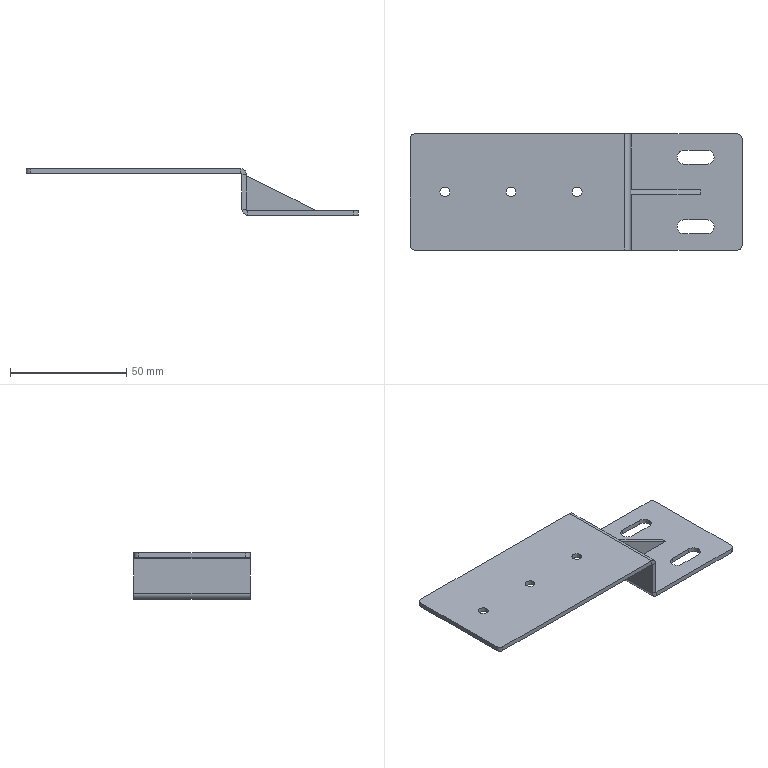Part | SolidWorks | features EdgeFlange 2, Fillet 1, FlatPattern 1, Gusset 1, HoleWzd 1, ICE 1, SMBaseFlange 1, SheetMetal 1 | 2 solids | 47 faces | box 143 x 50 x 20 mm | volume 15978 mm3 | plane 27 | cylinder 20 | commonest cylinder face diameters 4.2 x6 6 x6 4 x4 1 x2 5 x2
STEP:
#1=CARTESIAN_POINT('',(-23.,-1.,15.));
#2=VERTEX_POINT('',#1);
#3=CARTESIAN_POINT('',(7.,-1.,0.));
#4=VERTEX_POINT('',#3);
#5=CARTESIAN_POINT('',(-23.,-1.,15.));
#6=DIRECTION('',(0.8944,0.,-0.4472));
#7=VECTOR('',#6,1000.);
#8=LINE('',#5,#7);
#9=EDGE_CURVE('',#2,#4,#8,.T.);
#10=ORIENTED_EDGE('',*,*,#9,.T.);
#11=CARTESIAN_POINT('',(7.,1.,0.));
#12=VERTEX_POINT('',#11);
#13=CARTESIAN_POINT('',(7.,1.,0.));
#14=DIRECTION('',(0.,-1.,0.));
#15=VECTOR('',#14,1000.);
#16=LINE('',#13,#15);
#17=EDGE_CURVE('',#12,#4,#16,.T.);
#18=ORIENTED_EDGE('',*,*,#17,.F.);
#19=CARTESIAN_POINT('',(-23.,1.,15.));
#20=VERTEX_POINT('',#19);
#21=CARTESIAN_POINT('',(-23.,1.,15.));
#22=DIRECTION('',(0.8944,0.,-0.4472));
#23=VECTOR('',#22,1000.);
#24=LINE('',#21,#23);
#25=EDGE_CURVE('',#20,#12,#24,.T.);
#26=ORIENTED_EDGE('',*,*,#25,.F.);
#27=CARTESIAN_POINT('',(-23.,1.,15.));
#28=DIRECTION('',(0.,-1.,0.));
#29=VECTOR('',#28,1000.);
#30=LINE('',#27,#29);
#31=EDGE_CURVE('',#20,#2,#30,.T.);
#32=ORIENTED_EDGE('',*,*,#31,.T.);
#33=EDGE_LOOP('',(#10,#18,#26,#32));
#34=FACE_OUTER_BOUND('',#33,.T.);
#35=CARTESIAN_POINT('',(-23.,1.,15.));
#36=DIRECTION('',(-0.4472,0.,-0.8944));
#37=DIRECTION('',(-0.8944,0.,0.4472));
#38=AXIS2_PLACEMENT_3D('',#35,#36,#37);
#39=PLANE('',#38);
#40=ADVANCED_FACE('',(#34),#39,.F.);
#41=CARTESIAN_POINT('',(-23.,-1.,0.));
#42=VERTEX_POINT('',#41);
#43=CARTESIAN_POINT('',(-23.,-1.,0.));
#44=DIRECTION('',(-1.,0.,0.));
#45=VECTOR('',#44,1000.);
#46=LINE('',#43,#45);
#47=EDGE_CURVE('',#4,#42,#46,.T.);
#48=ORIENTED_EDGE('',*,*,#47,.T.);
#49=CARTESIAN_POINT('',(-23.,1.,0.));
#50=VERTEX_POINT('',#49);
#51=CARTESIAN_POINT('',(-23.,1.,0.));
#52=DIRECTION('',(0.,-1.,0.));
#53=VECTOR('',#52,1000.);
#54=LINE('',#51,#53);
#55=EDGE_CURVE('',#50,#42,#54,.T.);
#56=ORIENTED_EDGE('',*,*,#55,.F.);
#57=CARTESIAN_POINT('',(-23.,1.,0.));
#58=DIRECTION('',(-1.,0.,0.));
#59=VECTOR('',#58,1000.);
#60=LINE('',#57,#59);
#61=EDGE_CURVE('',#12,#50,#60,.T.);
#62=ORIENTED_EDGE('',*,*,#61,.F.);
#63=ORIENTED_EDGE('',*,*,#17,.T.);
#64=EDGE_LOOP('',(#48,#56,#62,#63));
#65=FACE_OUTER_BOUND('',#64,.T.);
#66=CARTESIAN_POINT('',(-23.,1.,0.));
#67=DIRECTION('',(0.,0.,1.));
#68=DIRECTION('',(1.,0.,0.));
#69=AXIS2_PLACEMENT_3D('',#66,#67,#68);
#70=PLANE('',#69);
#71=ADVANCED_FACE('',(#65),#70,.F.);
#72=CARTESIAN_POINT('',(-23.,-1.,0.));
#73=DIRECTION('',(0.,0.,1.));
#74=VECTOR('',#73,1000.);
#75=LINE('',#72,#74);
#76=EDGE_CURVE('',#42,#2,#75,.T.);
#77=ORIENTED_EDGE('',*,*,#76,.T.);
#78=ORIENTED_EDGE('',*,*,#31,.F.);
#79=CARTESIAN_POINT('',(-23.,1.,0.));
#80=DIRECTION('',(0.,0.,1.));
#81=VECTOR('',#80,1000.);
#82=LINE('',#79,#81);
#83=EDGE_CURVE('',#50,#20,#82,.T.);
#84=ORIENTED_EDGE('',*,*,#83,.F.);
#85=ORIENTED_EDGE('',*,*,#55,.T.);
#86=EDGE_LOOP('',(#77,#78,#84,#85));
#87=FACE_OUTER_BOUND('',#86,.T.);
#88=CARTESIAN_POINT('',(-23.,1.,0.));
#89=DIRECTION('',(1.,0.,0.));
#90=DIRECTION('',(0.,0.,-1.));
#91=AXIS2_PLACEMENT_3D('',#88,#89,#90);
#92=PLANE('',#91);
#93=ADVANCED_FACE('',(#87),#92,.F.);
#94=ORIENTED_EDGE('',*,*,#25,.T.);
#95=ORIENTED_EDGE('',*,*,#61,.T.);
#96=ORIENTED_EDGE('',*,*,#83,.T.);
#97=EDGE_LOOP('',(#94,#95,#96));
#98=FACE_OUTER_BOUND('',#97,.T.);
#99=CARTESIAN_POINT('',(0.,1.,0.));
#100=DIRECTION('',(0.,-1.,0.));
#101=DIRECTION('',(0.,0.,-1.));
#102=AXIS2_PLACEMENT_3D('',#99,#100,#101);
#103=PLANE('',#102);
#104=ADVANCED_FACE('',(#98),#103,.F.);
#105=ORIENTED_EDGE('',*,*,#9,.F.);
#106=ORIENTED_EDGE('',*,*,#76,.F.);
#107=ORIENTED_EDGE('',*,*,#47,.F.);
#108=EDGE_LOOP('',(#105,#106,#107));
#109=FACE_OUTER_BOUND('',#108,.T.);
#110=CARTESIAN_POINT('',(0.,-1.,0.));
#111=DIRECTION('',(0.,-1.,0.));
#112=DIRECTION('',(0.,0.,-1.));
#113=AXIS2_PLACEMENT_3D('',#110,#111,#112);
#114=PLANE('',#113);
#115=ADVANCED_FACE('',(#109),#114,.T.);
#116=CLOSED_SHELL('',(#40,#71,#93,#104,#115));
#117=MANIFOLD_SOLID_BREP('',#116);
#118=CARTESIAN_POINT('',(-105.1,0.,16.));
#119=VERTEX_POINT('',#118);
#120=CARTESIAN_POINT('',(-100.9,0.,16.));
#121=VERTEX_POINT('',#120);
#122=CARTESIAN_POINT('',(-103.,0.,16.));
#123=DIRECTION('',(0.,0.,1.));
#124=DIRECTION('',(1.,0.,0.));
#125=AXIS2_PLACEMENT_3D('',#122,#123,#124);
#126=CIRCLE('',#125,2.1);
#127=EDGE_CURVE('',#119,#121,#126,.T.);
#128=ORIENTED_EDGE('',*,*,#127,.F.);
#129=CARTESIAN_POINT('',(-105.1,0.,18.));
#130=VERTEX_POINT('',#129);
#131=CARTESIAN_POINT('',(-105.1,0.,18.));
#132=DIRECTION('',(0.,0.,1.));
#133=VECTOR('',#132,1000.);
#134=LINE('',#131,#133);
#135=EDGE_CURVE('',#119,#130,#134,.T.);
#136=ORIENTED_EDGE('',*,*,#135,.T.);
#137=CARTESIAN_POINT('',(-100.9,0.,18.));
#138=VERTEX_POINT('',#137);
#139=CARTESIAN_POINT('',(-103.,0.,18.));
#140=DIRECTION('',(0.,0.,1.));
#141=DIRECTION('',(1.,0.,0.));
#142=AXIS2_PLACEMENT_3D('',#139,#140,#141);
#143=CIRCLE('',#142,2.1);
#144=EDGE_CURVE('',#130,#138,#143,.T.);
#145=ORIENTED_EDGE('',*,*,#144,.T.);
#146=CARTESIAN_POINT('',(-100.9,0.,18.));
#147=DIRECTION('',(0.,0.,1.));
#148=VECTOR('',#147,1000.);
#149=LINE('',#146,#148);
#150=EDGE_CURVE('',#121,#138,#149,.T.);
#151=ORIENTED_EDGE('',*,*,#150,.F.);
#152=EDGE_LOOP('',(#128,#136,#145,#151));
#153=FACE_OUTER_BOUND('',#152,.T.);
#154=CARTESIAN_POINT('',(-103.,0.,18.));
#155=DIRECTION('',(0.,0.,1.));
#156=DIRECTION('',(1.,0.,0.));
#157=AXIS2_PLACEMENT_3D('',#154,#155,#156);
#158=CYLINDRICAL_SURFACE('',#157,2.1);
#159=ADVANCED_FACE('',(#153),#158,.F.);
#160=CARTESIAN_POINT('',(-76.6,0.,16.));
#161=VERTEX_POINT('',#160);
#162=CARTESIAN_POINT('',(-72.4,0.,16.));
#163=VERTEX_POINT('',#162);
#164=CARTESIAN_POINT('',(-74.5,0.,16.));
#165=DIRECTION('',(0.,0.,1.));
#166=DIRECTION('',(1.,0.,0.));
#167=AXIS2_PLACEMENT_3D('',#164,#165,#166);
#168=CIRCLE('',#167,2.1);
#169=EDGE_CURVE('',#161,#163,#168,.T.);
#170=ORIENTED_EDGE('',*,*,#169,.F.);
#171=CARTESIAN_POINT('',(-76.6,0.,18.));
#172=VERTEX_POINT('',#171);
#173=CARTESIAN_POINT('',(-76.6,0.,18.));
#174=DIRECTION('',(0.,0.,1.));
#175=VECTOR('',#174,1000.);
#176=LINE('',#173,#175);
#177=EDGE_CURVE('',#161,#172,#176,.T.);
#178=ORIENTED_EDGE('',*,*,#177,.T.);
#179=CARTESIAN_POINT('',(-72.4,0.,18.));
#180=VERTEX_POINT('',#179);
#181=CARTESIAN_POINT('',(-74.5,0.,18.));
#182=DIRECTION('',(0.,0.,1.));
#183=DIRECTION('',(1.,0.,0.));
#184=AXIS2_PLACEMENT_3D('',#181,#182,#183);
#185=CIRCLE('',#184,2.1);
#186=EDGE_CURVE('',#172,#180,#185,.T.);
#187=ORIENTED_EDGE('',*,*,#186,.T.);
#188=CARTESIAN_POINT('',(-72.4,0.,18.));
#189=DIRECTION('',(0.,0.,1.));
#190=VECTOR('',#189,1000.);
#191=LINE('',#188,#190);
#192=EDGE_CURVE('',#163,#180,#191,.T.);
#193=ORIENTED_EDGE('',*,*,#192,.F.);
#194=EDGE_LOOP('',(#170,#178,#187,#193));
#195=FACE_OUTER_BOUND('',#194,.T.);
#196=CARTESIAN_POINT('',(-74.5,0.,18.));
#197=DIRECTION('',(0.,0.,1.));
#198=DIRECTION('',(1.,0.,0.));
#199=AXIS2_PLACEMENT_3D('',#196,#197,#198);
#200=CYLINDRICAL_SURFACE('',#199,2.1);
#201=ADVANCED_FACE('',(#195),#200,.F.);
#202=CARTESIAN_POINT('',(-48.1,0.,16.));
#203=VERTEX_POINT('',#202);
#204=CARTESIAN_POINT('',(-43.9,0.,16.));
#205=VERTEX_POINT('',#204);
#206=CARTESIAN_POINT('',(-46.,0.,16.));
#207=DIRECTION('',(0.,0.,1.));
#208=DIRECTION('',(1.,0.,0.));
#209=AXIS2_PLACEMENT_3D('',#206,#207,#208);
#210=CIRCLE('',#209,2.1);
#211=EDGE_CURVE('',#203,#205,#210,.T.);
#212=ORIENTED_EDGE('',*,*,#211,.F.);
#213=CARTESIAN_POINT('',(-48.1,0.,18.));
#214=VERTEX_POINT('',#213);
#215=CARTESIAN_POINT('',(-48.1,0.,18.));
#216=DIRECTION('',(0.,0.,1.));
#217=VECTOR('',#216,1000.);
#218=LINE('',#215,#217);
#219=EDGE_CURVE('',#203,#214,#218,.T.);
#220=ORIENTED_EDGE('',*,*,#219,.T.);
#221=CARTESIAN_POINT('',(-43.9,0.,18.));
#222=VERTEX_POINT('',#221);
#223=CARTESIAN_POINT('',(-46.,0.,18.));
#224=DIRECTION('',(0.,0.,1.));
#225=DIRECTION('',(1.,0.,0.));
#226=AXIS2_PLACEMENT_3D('',#223,#224,#225);
#227=CIRCLE('',#226,2.1);
#228=EDGE_CURVE('',#214,#222,#227,.T.);
#229=ORIENTED_EDGE('',*,*,#228,.T.);
#230=CARTESIAN_POINT('',(-43.9,0.,18.));
#231=DIRECTION('',(0.,0.,1.));
#232=VECTOR('',#231,1000.);
#233=LINE('',#230,#232);
#234=EDGE_CURVE('',#205,#222,#233,.T.);
#235=ORIENTED_EDGE('',*,*,#234,.F.);
#236=EDGE_LOOP('',(#212,#220,#229,#235));
#237=FACE_OUTER_BOUND('',#236,.T.);
#238=CARTESIAN_POINT('',(-46.,0.,18.));
#239=DIRECTION('',(0.,0.,1.));
#240=DIRECTION('',(1.,0.,0.));
#241=AXIS2_PLACEMENT_3D('',#238,#239,#240);
#242=CYLINDRICAL_SURFACE('',#241,2.1);
#243=ADVANCED_FACE('',(#237),#242,.F.);
#244=CARTESIAN_POINT('',(10.,-12.,-2.));
#245=VERTEX_POINT('',#244);
#246=CARTESIAN_POINT('',(13.,-15.,-2.));
#247=VERTEX_POINT('',#246);
#248=CARTESIAN_POINT('',(10.,-15.,-2.));
#249=DIRECTION('',(0.,0.,-1.));
#250=DIRECTION('',(1.,0.,0.));
#251=AXIS2_PLACEMENT_3D('',#248,#249,#250);
#252=CIRCLE('',#251,3.);
#253=EDGE_CURVE('',#245,#247,#252,.T.);
#254=ORIENTED_EDGE('',*,*,#253,.T.);
#255=CARTESIAN_POINT('',(13.,-15.,0.));
#256=VERTEX_POINT('',#255);
#257=CARTESIAN_POINT('',(13.,-15.,-2.001));
#258=DIRECTION('',(0.,0.,1.));
#259=VECTOR('',#258,1000.);
#260=LINE('',#257,#259);
#261=EDGE_CURVE('',#247,#256,#260,.T.);
#262=ORIENTED_EDGE('',*,*,#261,.T.);
#263=CARTESIAN_POINT('',(10.,-12.,0.));
#264=VERTEX_POINT('',#263);
#265=CARTESIAN_POINT('',(10.,-15.,0.));
#266=DIRECTION('',(0.,0.,1.));
#267=DIRECTION('',(1.,0.,0.));
#268=AXIS2_PLACEMENT_3D('',#265,#266,#267);
#269=CIRCLE('',#268,3.);
#270=EDGE_CURVE('',#256,#264,#269,.T.);
#271=ORIENTED_EDGE('',*,*,#270,.T.);
#272=CARTESIAN_POINT('',(10.,-12.,-2.001));
#273=DIRECTION('',(0.,0.,1.));
#274=VECTOR('',#273,1000.);
#275=LINE('',#272,#274);
#276=EDGE_CURVE('',#245,#264,#275,.T.);
#277=ORIENTED_EDGE('',*,*,#276,.F.);
#278=EDGE_LOOP('',(#254,#262,#271,#277));
#279=FACE_OUTER_BOUND('',#278,.T.);
#280=CARTESIAN_POINT('',(10.,-15.,-2.001));
#281=DIRECTION('',(0.,0.,1.));
#282=DIRECTION('',(1.,0.,0.));
#283=AXIS2_PLACEMENT_3D('',#280,#281,#282);
#284=CYLINDRICAL_SURFACE('',#283,3.);
#285=ADVANCED_FACE('',(#279),#284,.F.);
#286=CARTESIAN_POINT('',(10.,18.,-2.));
#287=VERTEX_POINT('',#286);
#288=CARTESIAN_POINT('',(13.,15.,-2.));
#289=VERTEX_POINT('',#288);
#290=CARTESIAN_POINT('',(10.,15.,-2.));
#291=DIRECTION('',(0.,0.,-1.));
#292=DIRECTION('',(1.,0.,0.));
#293=AXIS2_PLACEMENT_3D('',#290,#291,#292);
#294=CIRCLE('',#293,3.);
#295=EDGE_CURVE('',#287,#289,#294,.T.);
#296=ORIENTED_EDGE('',*,*,#295,.T.);
#297=CARTESIAN_POINT('',(13.,15.,0.));
#298=VERTEX_POINT('',#297);
#299=CARTESIAN_POINT('',(13.,15.,-2.001));
#300=DIRECTION('',(0.,0.,1.));
#301=VECTOR('',#300,1000.);
#302=LINE('',#299,#301);
#303=EDGE_CURVE('',#289,#298,#302,.T.);
#304=ORIENTED_EDGE('',*,*,#303,.T.);
#305=CARTESIAN_POINT('',(10.,18.,0.));
#306=VERTEX_POINT('',#305);
#307=CARTESIAN_POINT('',(10.,15.,0.));
#308=DIRECTION('',(0.,0.,1.));
#309=DIRECTION('',(1.,0.,0.));
#310=AXIS2_PLACEMENT_3D('',#307,#308,#309);
#311=CIRCLE('',#310,3.);
#312=EDGE_CURVE('',#298,#306,#311,.T.);
#313=ORIENTED_EDGE('',*,*,#312,.T.);
#314=CARTESIAN_POINT('',(10.,18.,-2.001));
#315=DIRECTION('',(0.,0.,1.));
#316=VECTOR('',#315,1000.);
#317=LINE('',#314,#316);
#318=EDGE_CURVE('',#287,#306,#317,.T.);
#319=ORIENTED_EDGE('',*,*,#318,.F.);
#320=EDGE_LOOP('',(#296,#304,#313,#319));
#321=FACE_OUTER_BOUND('',#320,.T.);
#322=CARTESIAN_POINT('',(10.,15.,-2.001));
#323=DIRECTION('',(0.,0.,1.));
#324=DIRECTION('',(1.,0.,0.));
#325=AXIS2_PLACEMENT_3D('',#322,#323,#324);
#326=CYLINDRICAL_SURFACE('',#325,3.);
#327=ADVANCED_FACE('',(#321),#326,.F.);
#328=CARTESIAN_POINT('',(-25.,25.,15.5));
#329=VERTEX_POINT('',#328);
#330=CARTESIAN_POINT('',(-23.,25.,15.5));
#331=VERTEX_POINT('',#330);
#332=CARTESIAN_POINT('',(-25.,25.,15.5));
#333=DIRECTION('',(1.,0.,0.));
#334=VECTOR('',#333,1000.);
#335=LINE('',#332,#334);
#336=EDGE_CURVE('',#329,#331,#335,.T.);
#337=ORIENTED_EDGE('',*,*,#336,.T.);
#338=CARTESIAN_POINT('',(-23.,25.,0.5));
#339=VERTEX_POINT('',#338);
#340=CARTESIAN_POINT('',(-23.,25.,0.));
#341=DIRECTION('',(0.,0.,-1.));
#342=VECTOR('',#341,1000.);
#343=LINE('',#340,#342);
#344=EDGE_CURVE('',#331,#339,#343,.T.);
#345=ORIENTED_EDGE('',*,*,#344,.T.);
#346=CARTESIAN_POINT('',(-25.,25.,0.5));
#347=VERTEX_POINT('',#346);
#348=CARTESIAN_POINT('',(-25.,25.,0.5));
#349=DIRECTION('',(-1.,0.,0.));
#350=VECTOR('',#349,1000.);
#351=LINE('',#348,#350);
#352=EDGE_CURVE('',#339,#347,#351,.T.);
#353=ORIENTED_EDGE('',*,*,#352,.T.);
#354=CARTESIAN_POINT('',(-25.,25.,0.));
#355=DIRECTION('',(0.,0.,-1.));
#356=VECTOR('',#355,1000.);
#357=LINE('',#354,#356);
#358=EDGE_CURVE('',#329,#347,#357,.T.);
#359=ORIENTED_EDGE('',*,*,#358,.F.);
#360=EDGE_LOOP('',(#337,#345,#353,#359));
#361=FACE_OUTER_BOUND('',#360,.T.);
#362=CARTESIAN_POINT('',(-25.,25.,0.));
#363=DIRECTION('',(0.,-1.,0.));
#364=DIRECTION('',(0.,0.,-1.));
#365=AXIS2_PLACEMENT_3D('',#362,#363,#364);
#366=PLANE('',#365);
#367=ADVANCED_FACE('',(#361),#366,.F.);
#368=CARTESIAN_POINT('',(-25.,-25.,15.5));
#369=VERTEX_POINT('',#368);
#370=CARTESIAN_POINT('',(-23.,-25.,15.5));
#371=VERTEX_POINT('',#370);
#372=CARTESIAN_POINT('',(-25.,-25.,15.5));
#373=DIRECTION('',(1.,0.,0.));
#374=VECTOR('',#373,1000.);
#375=LINE('',#372,#374);
#376=EDGE_CURVE('',#369,#371,#375,.T.);
#377=ORIENTED_EDGE('',*,*,#376,.F.);
#378=CARTESIAN_POINT('',(-25.,-25.,0.5));
#379=VERTEX_POINT('',#378);
#380=CARTESIAN_POINT('',(-25.,-25.,0.));
#381=DIRECTION('',(0.,0.,1.));
#382=VECTOR('',#381,1000.);
#383=LINE('',#380,#382);
#384=EDGE_CURVE('',#379,#369,#383,.T.);
#385=ORIENTED_EDGE('',*,*,#384,.F.);
#386=CARTESIAN_POINT('',(-23.,-25.,0.5));
#387=VERTEX_POINT('',#386);
#388=CARTESIAN_POINT('',(-23.,-25.,0.5));
#389=DIRECTION('',(-1.,0.,0.));
#390=VECTOR('',#389,1000.);
#391=LINE('',#388,#390);
#392=EDGE_CURVE('',#387,#379,#391,.T.);
#393=ORIENTED_EDGE('',*,*,#392,.F.);
#394=CARTESIAN_POINT('',(-23.,-25.,18.));
#395=DIRECTION('',(0.,0.,1.));
#396=VECTOR('',#395,1000.);
#397=LINE('',#394,#396);
#398=EDGE_CURVE('',#387,#371,#397,.T.);
#399=ORIENTED_EDGE('',*,*,#398,.T.);
#400=EDGE_LOOP('',(#377,#385,#393,#399));
#401=FACE_OUTER_BOUND('',#400,.T.);
#402=CARTESIAN_POINT('',(-25.,-25.,18.));
#403=DIRECTION('',(0.,1.,0.));
#404=DIRECTION('',(0.,0.,1.));
#405=AXIS2_PLACEMENT_3D('',#402,#403,#404);
#406=PLANE('',#405);
#407=ADVANCED_FACE('',(#401),#406,.F.);
#408=CARTESIAN_POINT('',(-25.,25.,15.5));
#409=DIRECTION('',(0.,-1.,0.));
#410=VECTOR('',#409,1000.);
#411=LINE('',#408,#410);
#412=EDGE_CURVE('',#329,#369,#411,.T.);
#413=ORIENTED_EDGE('',*,*,#412,.F.);
#414=ORIENTED_EDGE('',*,*,#358,.T.);
#415=CARTESIAN_POINT('',(-25.,25.,0.5));
#416=DIRECTION('',(0.,1.,0.));
#417=VECTOR('',#416,1000.);
#418=LINE('',#415,#417);
#419=EDGE_CURVE('',#379,#347,#418,.T.);
#420=ORIENTED_EDGE('',*,*,#419,.F.);
#421=ORIENTED_EDGE('',*,*,#384,.T.);
#422=EDGE_LOOP('',(#413,#414,#420,#421));
#423=FACE_OUTER_BOUND('',#422,.T.);
#424=CARTESIAN_POINT('',(-25.,0.,0.));
#425=DIRECTION('',(1.,0.,0.));
#426=DIRECTION('',(0.,0.,-1.));
#427=AXIS2_PLACEMENT_3D('',#424,#425,#426);
#428=PLANE('',#427);
#429=ADVANCED_FACE('',(#423),#428,.F.);
#430=ORIENTED_EDGE('',*,*,#344,.F.);
#431=CARTESIAN_POINT('',(-23.,25.,15.5));
#432=DIRECTION('',(0.,-1.,0.));
#433=VECTOR('',#432,1000.);
#434=LINE('',#431,#433);
#435=EDGE_CURVE('',#331,#371,#434,.T.);
#436=ORIENTED_EDGE('',*,*,#435,.T.);
#437=ORIENTED_EDGE('',*,*,#398,.F.);
#438=CARTESIAN_POINT('',(-23.,25.,0.5));
#439=DIRECTION('',(0.,-1.,0.));
#440=VECTOR('',#439,1000.);
#441=LINE('',#438,#440);
#442=EDGE_CURVE('',#339,#387,#441,.T.);
#443=ORIENTED_EDGE('',*,*,#442,.F.);
#444=EDGE_LOOP('',(#430,#436,#437,#443));
#445=FACE_OUTER_BOUND('',#444,.T.);
#446=CARTESIAN_POINT('',(-23.,0.,0.));
#447=DIRECTION('',(1.,0.,0.));
#448=DIRECTION('',(0.,0.,-1.));
#449=AXIS2_PLACEMENT_3D('',#446,#447,#448);
#450=PLANE('',#449);
#451=ADVANCED_FACE('',(#445),#450,.T.);
#452=CARTESIAN_POINT('',(-22.5,-25.,-2.));
#453=VERTEX_POINT('',#452);
#454=CARTESIAN_POINT('',(23.,-25.,-2.));
#455=VERTEX_POINT('',#454);
#456=CARTESIAN_POINT('',(25.,-25.,-2.));
#457=DIRECTION('',(1.,0.,0.));
#458=VECTOR('',#457,1000.);
#459=LINE('',#456,#458);
#460=EDGE_CURVE('',#453,#455,#459,.T.);
#461=ORIENTED_EDGE('',*,*,#460,.T.);
#462=CARTESIAN_POINT('',(23.,-25.,0.));
#463=VERTEX_POINT('',#462);
#464=CARTESIAN_POINT('',(23.,-25.,-2.));
#465=DIRECTION('',(0.,0.,1.));
#466=VECTOR('',#465,1000.);
#467=LINE('',#464,#466);
#468=EDGE_CURVE('',#455,#463,#467,.T.);
#469=ORIENTED_EDGE('',*,*,#468,.T.);
#470=CARTESIAN_POINT('',(-22.5,-25.,0.));
#471=VERTEX_POINT('',#470);
#472=CARTESIAN_POINT('',(25.,-25.,0.));
#473=DIRECTION('',(1.,0.,0.));
#474=VECTOR('',#473,1000.);
#475=LINE('',#472,#474);
#476=EDGE_CURVE('',#471,#463,#475,.T.);
#477=ORIENTED_EDGE('',*,*,#476,.F.);
#478=CARTESIAN_POINT('',(-22.5,-25.,0.));
#479=DIRECTION('',(0.,0.,-1.));
#480=VECTOR('',#479,1000.);
#481=LINE('',#478,#480);
#482=EDGE_CURVE('',#471,#453,#481,.T.);
#483=ORIENTED_EDGE('',*,*,#482,.T.);
#484=EDGE_LOOP('',(#461,#469,#477,#483));
#485=FACE_OUTER_BOUND('',#484,.T.);
#486=CARTESIAN_POINT('',(25.,-25.,-2.));
#487=DIRECTION('',(0.,-1.,0.));
#488=DIRECTION('',(0.,0.,-1.));
#489=AXIS2_PLACEMENT_3D('',#486,#487,#488);
#490=PLANE('',#489);
#491=ADVANCED_FACE('',(#485),#490,.T.);
#492=CARTESIAN_POINT('',(0.,-12.,-2.));
#493=VERTEX_POINT('',#492);
#494=CARTESIAN_POINT('',(0.,-12.,-2.));
#495=DIRECTION('',(1.,0.,0.));
#496=VECTOR('',#495,1000.);
#497=LINE('',#494,#496);
#498=EDGE_CURVE('',#493,#245,#497,.T.);
#499=ORIENTED_EDGE('',*,*,#498,.F.);
#500=CARTESIAN_POINT('',(0.,-18.,-2.));
#501=VERTEX_POINT('',#500);
#502=CARTESIAN_POINT('',(0.,-15.,-2.));
#503=DIRECTION('',(0.,0.,-1.));
#504=DIRECTION('',(1.,0.,0.));
#505=AXIS2_PLACEMENT_3D('',#502,#503,#504);
#506=CIRCLE('',#505,3.);
#507=EDGE_CURVE('',#501,#493,#506,.T.);
#508=ORIENTED_EDGE('',*,*,#507,.F.);
#509=CARTESIAN_POINT('',(10.,-18.,-2.));
#510=VERTEX_POINT('',#509);
#511=CARTESIAN_POINT('',(0.,-18.,-2.));
#512=DIRECTION('',(-1.,0.,0.));
#513=VECTOR('',#512,1000.);
#514=LINE('',#511,#513);
#515=EDGE_CURVE('',#510,#501,#514,.T.);
#516=ORIENTED_EDGE('',*,*,#515,.F.);
#517=CARTESIAN_POINT('',(10.,-15.,-2.));
#518=DIRECTION('',(0.,0.,-1.));
#519=DIRECTION('',(1.,0.,0.));
#520=AXIS2_PLACEMENT_3D('',#517,#518,#519);
#521=CIRCLE('',#520,3.);
#522=EDGE_CURVE('',#247,#510,#521,.T.);
#523=ORIENTED_EDGE('',*,*,#522,.F.);
#524=ORIENTED_EDGE('',*,*,#253,.F.);
#525=EDGE_LOOP('',(#499,#508,#516,#523,#524));
#526=FACE_BOUND('',#525,.T.);
#527=CARTESIAN_POINT('',(0.,18.,-2.));
#528=VERTEX_POINT('',#527);
#529=CARTESIAN_POINT('',(0.,18.,-2.));
#530=DIRECTION('',(1.,0.,0.));
#531=VECTOR('',#530,1000.);
#532=LINE('',#529,#531);
#533=EDGE_CURVE('',#528,#287,#532,.T.);
#534=ORIENTED_EDGE('',*,*,#533,.F.);
#535=CARTESIAN_POINT('',(0.,12.,-2.));
#536=VERTEX_POINT('',#535);
#537=CARTESIAN_POINT('',(0.,15.,-2.));
#538=DIRECTION('',(0.,0.,-1.));
#539=DIRECTION('',(1.,0.,0.));
#540=AXIS2_PLACEMENT_3D('',#537,#538,#539);
#541=CIRCLE('',#540,3.);
#542=EDGE_CURVE('',#536,#528,#541,.T.);
#543=ORIENTED_EDGE('',*,*,#542,.F.);
#544=CARTESIAN_POINT('',(10.,12.,-2.));
#545=VERTEX_POINT('',#544);
#546=CARTESIAN_POINT('',(0.,12.,-2.));
#547=DIRECTION('',(-1.,0.,0.));
#548=VECTOR('',#547,1000.);
#549=LINE('',#546,#548);
#550=EDGE_CURVE('',#545,#536,#549,.T.);
#551=ORIENTED_EDGE('',*,*,#550,.F.);
#552=CARTESIAN_POINT('',(10.,15.,-2.));
#553=DIRECTION('',(0.,0.,-1.));
#554=DIRECTION('',(1.,0.,0.));
#555=AXIS2_PLACEMENT_3D('',#552,#553,#554);
#556=CIRCLE('',#555,3.);
#557=EDGE_CURVE('',#289,#545,#556,.T.);
#558=ORIENTED_EDGE('',*,*,#557,.F.);
#559=ORIENTED_EDGE('',*,*,#295,.F.);
#560=EDGE_LOOP('',(#534,#543,#551,#558,#559));
#561=FACE_BOUND('',#560,.T.);
#562=CARTESIAN_POINT('',(25.,-23.,-2.));
#563=VERTEX_POINT('',#562);
#564=CARTESIAN_POINT('',(25.,23.,-2.));
#565=VERTEX_POINT('',#564);
#566=CARTESIAN_POINT('',(25.,-25.,-2.));
#567=DIRECTION('',(0.,1.,0.));
#568=VECTOR('',#567,1000.);
#569=LINE('',#566,#568);
#570=EDGE_CURVE('',#563,#565,#569,.T.);
#571=ORIENTED_EDGE('',*,*,#570,.F.);
#572=CARTESIAN_POINT('',(23.,-23.,-2.));
#573=DIRECTION('',(0.,0.,-1.));
#574=DIRECTION('',(1.,0.,0.));
#575=AXIS2_PLACEMENT_3D('',#572,#573,#574);
#576=CIRCLE('',#575,2.);
#577=EDGE_CURVE('',#563,#455,#576,.T.);
#578=ORIENTED_EDGE('',*,*,#577,.T.);
#579=ORIENTED_EDGE('',*,*,#460,.F.);
#580=CARTESIAN_POINT('',(-22.5,25.,-2.));
#581=VERTEX_POINT('',#580);
#582=CARTESIAN_POINT('',(-22.5,-25.,-2.));
#583=DIRECTION('',(0.,1.,0.));
#584=VECTOR('',#583,1000.);
#585=LINE('',#582,#584);
#586=EDGE_CURVE('',#453,#581,#585,.T.);
#587=ORIENTED_EDGE('',*,*,#586,.T.);
#588=CARTESIAN_POINT('',(23.,25.,-2.));
#589=VERTEX_POINT('',#588);
#590=CARTESIAN_POINT('',(25.,25.,-2.));
#591=DIRECTION('',(-1.,0.,0.));
#592=VECTOR('',#591,1000.);
#593=LINE('',#590,#592);
#594=EDGE_CURVE('',#589,#581,#593,.T.);
#595=ORIENTED_EDGE('',*,*,#594,.F.);
#596=CARTESIAN_POINT('',(23.,23.,-2.));
#597=DIRECTION('',(0.,0.,-1.));
#598=DIRECTION('',(1.,0.,0.));
#599=AXIS2_PLACEMENT_3D('',#596,#597,#598);
#600=CIRCLE('',#599,2.);
#601=EDGE_CURVE('',#589,#565,#600,.T.);
#602=ORIENTED_EDGE('',*,*,#601,.T.);
#603=EDGE_LOOP('',(#571,#578,#579,#587,#595,#602));
#604=FACE_OUTER_BOUND('',#603,.T.);
#605=CARTESIAN_POINT('',(0.,0.,-2.));
#606=DIRECTION('',(0.,0.,1.));
#607=DIRECTION('',(1.,0.,0.));
#608=AXIS2_PLACEMENT_3D('',#605,#606,#607);
#609=PLANE('',#608);
#610=ADVANCED_FACE('',(#526,#561,#604),#609,.F.);
#611=CARTESIAN_POINT('',(0.,-12.,0.));
#612=VERTEX_POINT('',#611);
#613=CARTESIAN_POINT('',(0.,-18.,0.));
#614=VERTEX_POINT('',#613);
#615=CARTESIAN_POINT('',(0.,-15.,0.));
#616=DIRECTION('',(0.,0.,1.));
#617=DIRECTION('',(1.,0.,0.));
#618=AXIS2_PLACEMENT_3D('',#615,#616,#617);
#619=CIRCLE('',#618,3.);
#620=EDGE_CURVE('',#612,#614,#619,.T.);
#621=ORIENTED_EDGE('',*,*,#620,.F.);
#622=CARTESIAN_POINT('',(0.,-12.,0.));
#623=DIRECTION('',(-1.,0.,0.));
#624=VECTOR('',#623,1000.);
#625=LINE('',#622,#624);
#626=EDGE_CURVE('',#264,#612,#625,.T.);
#627=ORIENTED_EDGE('',*,*,#626,.F.);
#628=ORIENTED_EDGE('',*,*,#270,.F.);
#629=CARTESIAN_POINT('',(10.,-18.,0.));
#630=VERTEX_POINT('',#629);
#631=CARTESIAN_POINT('',(10.,-15.,0.));
#632=DIRECTION('',(0.,0.,1.));
#633=DIRECTION('',(1.,0.,0.));
#634=AXIS2_PLACEMENT_3D('',#631,#632,#633);
#635=CIRCLE('',#634,3.);
#636=EDGE_CURVE('',#630,#256,#635,.T.);
#637=ORIENTED_EDGE('',*,*,#636,.F.);
#638=CARTESIAN_POINT('',(0.,-18.,0.));
#639=DIRECTION('',(1.,0.,0.));
#640=VECTOR('',#639,1000.);
#641=LINE('',#638,#640);
#642=EDGE_CURVE('',#614,#630,#641,.T.);
#643=ORIENTED_EDGE('',*,*,#642,.F.);
#644=EDGE_LOOP('',(#621,#627,#628,#637,#643));
#645=FACE_BOUND('',#644,.T.);
#646=CARTESIAN_POINT('',(0.,18.,0.));
#647=VERTEX_POINT('',#646);
#648=CARTESIAN_POINT('',(0.,12.,0.));
#649=VERTEX_POINT('',#648);
#650=CARTESIAN_POINT('',(0.,15.,0.));
#651=DIRECTION('',(0.,0.,1.));
#652=DIRECTION('',(1.,0.,0.));
#653=AXIS2_PLACEMENT_3D('',#650,#651,#652);
#654=CIRCLE('',#653,3.);
#655=EDGE_CURVE('',#647,#649,#654,.T.);
#656=ORIENTED_EDGE('',*,*,#655,.F.);
#657=CARTESIAN_POINT('',(0.,18.,0.));
#658=DIRECTION('',(-1.,0.,0.));
#659=VECTOR('',#658,1000.);
#660=LINE('',#657,#659);
#661=EDGE_CURVE('',#306,#647,#660,.T.);
#662=ORIENTED_EDGE('',*,*,#661,.F.);
#663=ORIENTED_EDGE('',*,*,#312,.F.);
#664=CARTESIAN_POINT('',(10.,12.,0.));
#665=VERTEX_POINT('',#664);
#666=CARTESIAN_POINT('',(10.,15.,0.));
#667=DIRECTION('',(0.,0.,1.));
#668=DIRECTION('',(1.,0.,0.));
#669=AXIS2_PLACEMENT_3D('',#666,#667,#668);
#670=CIRCLE('',#669,3.);
#671=EDGE_CURVE('',#665,#298,#670,.T.);
#672=ORIENTED_EDGE('',*,*,#671,.F.);
#673=CARTESIAN_POINT('',(0.,12.,0.));
#674=DIRECTION('',(1.,0.,0.));
#675=VECTOR('',#674,1000.);
#676=LINE('',#673,#675);
#677=EDGE_CURVE('',#649,#665,#676,.T.);
#678=ORIENTED_EDGE('',*,*,#677,.F.);
#679=EDGE_LOOP('',(#656,#662,#663,#672,#678));
#680=FACE_BOUND('',#679,.T.);
#681=ORIENTED_EDGE('',*,*,#476,.T.);
#682=CARTESIAN_POINT('',(25.,-23.,0.));
#683=VERTEX_POINT('',#682);
#684=CARTESIAN_POINT('',(23.,-23.,0.));
#685=DIRECTION('',(0.,0.,1.));
#686=DIRECTION('',(1.,0.,0.));
#687=AXIS2_PLACEMENT_3D('',#684,#685,#686);
#688=CIRCLE('',#687,2.);
#689=EDGE_CURVE('',#463,#683,#688,.T.);
#690=ORIENTED_EDGE('',*,*,#689,.T.);
#691=CARTESIAN_POINT('',(25.,23.,0.));
#692=VERTEX_POINT('',#691);
#693=CARTESIAN_POINT('',(25.,-25.,0.));
#694=DIRECTION('',(0.,1.,0.));
#695=VECTOR('',#694,1000.);
#696=LINE('',#693,#695);
#697=EDGE_CURVE('',#683,#692,#696,.T.);
#698=ORIENTED_EDGE('',*,*,#697,.T.);
#699=CARTESIAN_POINT('',(23.,25.,0.));
#700=VERTEX_POINT('',#699);
#701=CARTESIAN_POINT('',(23.,23.,0.));
#702=DIRECTION('',(0.,0.,1.));
#703=DIRECTION('',(1.,0.,0.));
#704=AXIS2_PLACEMENT_3D('',#701,#702,#703);
#705=CIRCLE('',#704,2.);
#706=EDGE_CURVE('',#692,#700,#705,.T.);
#707=ORIENTED_EDGE('',*,*,#706,.T.);
#708=CARTESIAN_POINT('',(-22.5,25.,0.));
#709=VERTEX_POINT('',#708);
#710=CARTESIAN_POINT('',(25.,25.,0.));
#711=DIRECTION('',(-1.,0.,0.));
#712=VECTOR('',#711,1000.);
#713=LINE('',#710,#712);
#714=EDGE_CURVE('',#700,#709,#713,.T.);
#715=ORIENTED_EDGE('',*,*,#714,.T.);
#716=CARTESIAN_POINT('',(-22.5,-25.,0.));
#717=DIRECTION('',(0.,1.,0.));
#718=VECTOR('',#717,1000.);
#719=LINE('',#716,#718);
#720=EDGE_CURVE('',#471,#709,#719,.T.);
#721=ORIENTED_EDGE('',*,*,#720,.F.);
#722=EDGE_LOOP('',(#681,#690,#698,#707,#715,#721));
#723=FACE_OUTER_BOUND('',#722,.T.);
#724=CARTESIAN_POINT('',(0.,0.,0.));
#725=DIRECTION('',(0.,0.,1.));
#726=DIRECTION('',(1.,0.,0.));
#727=AXIS2_PLACEMENT_3D('',#724,#725,#726);
#728=PLANE('',#727);
#729=ADVANCED_FACE('',(#645,#680,#723),#728,.T.);
#730=ORIENTED_EDGE('',*,*,#714,.F.);
#731=CARTESIAN_POINT('',(23.,25.,-2.));
#732=DIRECTION('',(0.,0.,-1.));
#733=VECTOR('',#732,1000.);
#734=LINE('',#731,#733);
#735=EDGE_CURVE('',#700,#589,#734,.T.);
#736=ORIENTED_EDGE('',*,*,#735,.T.);
#737=ORIENTED_EDGE('',*,*,#594,.T.);
#738=CARTESIAN_POINT('',(-22.5,25.,0.));
#739=DIRECTION('',(0.,0.,-1.));
#740=VECTOR('',#739,1000.);
#741=LINE('',#738,#740);
#742=EDGE_CURVE('',#709,#581,#741,.T.);
#743=ORIENTED_EDGE('',*,*,#742,.F.);
#744=EDGE_LOOP('',(#730,#736,#737,#743));
#745=FACE_OUTER_BOUND('',#744,.T.);
#746=CARTESIAN_POINT('',(25.,25.,-2.));
#747=DIRECTION('',(0.,1.,0.));
#748=DIRECTION('',(0.,0.,1.));
#749=AXIS2_PLACEMENT_3D('',#746,#747,#748);
#750=PLANE('',#749);
#751=ADVANCED_FACE('',(#745),#750,.T.);
#752=ORIENTED_EDGE('',*,*,#697,.F.);
#753=CARTESIAN_POINT('',(25.,-23.,-2.));
#754=DIRECTION('',(0.,0.,-1.));
#755=VECTOR('',#754,1000.);
#756=LINE('',#753,#755);
#757=EDGE_CURVE('',#683,#563,#756,.T.);
#758=ORIENTED_EDGE('',*,*,#757,.T.);
#759=ORIENTED_EDGE('',*,*,#570,.T.);
#760=CARTESIAN_POINT('',(25.,23.,-2.));
#761=DIRECTION('',(0.,0.,1.));
#762=VECTOR('',#761,1000.);
#763=LINE('',#760,#762);
#764=EDGE_CURVE('',#565,#692,#763,.T.);
#765=ORIENTED_EDGE('',*,*,#764,.T.);
#766=EDGE_LOOP('',(#752,#758,#759,#765));
#767=FACE_OUTER_BOUND('',#766,.T.);
#768=CARTESIAN_POINT('',(25.,-25.,-2.));
#769=DIRECTION('',(1.,0.,0.));
#770=DIRECTION('',(0.,0.,-1.));
#771=AXIS2_PLACEMENT_3D('',#768,#769,#770);
#772=PLANE('',#771);
#773=ADVANCED_FACE('',(#767),#772,.T.);
#774=ORIENTED_EDGE('',*,*,#352,.F.);
#775=CARTESIAN_POINT('',(-22.5,25.,0.5));
#776=DIRECTION('',(0.,1.,0.));
#777=DIRECTION('',(0.,0.,-1.));
#778=AXIS2_PLACEMENT_3D('',#775,#776,#777);
#779=CIRCLE('',#778,0.5);
#780=EDGE_CURVE('',#709,#339,#779,.T.);
#781=ORIENTED_EDGE('',*,*,#780,.F.);
#782=ORIENTED_EDGE('',*,*,#742,.T.);
#783=CARTESIAN_POINT('',(-22.5,25.,0.5));
#784=DIRECTION('',(0.,1.,0.));
#785=DIRECTION('',(0.,0.,-1.));
#786=AXIS2_PLACEMENT_3D('',#783,#784,#785);
#787=CIRCLE('',#786,2.5);
#788=EDGE_CURVE('',#581,#347,#787,.T.);
#789=ORIENTED_EDGE('',*,*,#788,.T.);
#790=EDGE_LOOP('',(#774,#781,#782,#789));
#791=FACE_OUTER_BOUND('',#790,.T.);
#792=CARTESIAN_POINT('',(-22.5,25.,0.5));
#793=DIRECTION('',(0.,1.,0.));
#794=DIRECTION('',(0.,0.,1.));
#795=AXIS2_PLACEMENT_3D('',#792,#793,#794);
#796=PLANE('',#795);
#797=ADVANCED_FACE('',(#791),#796,.T.);
#798=CARTESIAN_POINT('',(-22.5,-25.,0.5));
#799=DIRECTION('',(0.,-1.,0.));
#800=DIRECTION('',(0.,0.,-1.));
#801=AXIS2_PLACEMENT_3D('',#798,#799,#800);
#802=CIRCLE('',#801,0.5);
#803=EDGE_CURVE('',#387,#471,#802,.T.);
#804=ORIENTED_EDGE('',*,*,#803,.F.);
#805=ORIENTED_EDGE('',*,*,#392,.T.);
#806=CARTESIAN_POINT('',(-22.5,-25.,0.5));
#807=DIRECTION('',(0.,-1.,0.));
#808=DIRECTION('',(0.,0.,-1.));
#809=AXIS2_PLACEMENT_3D('',#806,#807,#808);
#810=CIRCLE('',#809,2.5);
#811=EDGE_CURVE('',#379,#453,#810,.T.);
#812=ORIENTED_EDGE('',*,*,#811,.T.);
#813=ORIENTED_EDGE('',*,*,#482,.F.);
#814=EDGE_LOOP('',(#804,#805,#812,#813));
#815=FACE_OUTER_BOUND('',#814,.T.);
#816=CARTESIAN_POINT('',(-22.5,-25.,0.5));
#817=DIRECTION('',(0.,1.,0.));
#818=DIRECTION('',(0.,0.,1.));
#819=AXIS2_PLACEMENT_3D('',#816,#817,#818);
#820=PLANE('',#819);
#821=ADVANCED_FACE('',(#815),#820,.F.);
#822=ORIENTED_EDGE('',*,*,#586,.F.);
#823=ORIENTED_EDGE('',*,*,#811,.F.);
#824=ORIENTED_EDGE('',*,*,#419,.T.);
#825=ORIENTED_EDGE('',*,*,#788,.F.);
#826=EDGE_LOOP('',(#822,#823,#824,#825));
#827=FACE_OUTER_BOUND('',#826,.T.);
#828=CARTESIAN_POINT('',(-22.5,-25.,0.5));
#829=DIRECTION('',(0.,-1.,0.));
#830=DIRECTION('',(-1.,0.,0.));
#831=AXIS2_PLACEMENT_3D('',#828,#829,#830);
#832=CYLINDRICAL_SURFACE('',#831,2.5);
#833=ADVANCED_FACE('',(#827),#832,.T.);
#834=ORIENTED_EDGE('',*,*,#720,.T.);
#835=ORIENTED_EDGE('',*,*,#780,.T.);
#836=ORIENTED_EDGE('',*,*,#442,.T.);
#837=ORIENTED_EDGE('',*,*,#803,.T.);
#838=EDGE_LOOP('',(#834,#835,#836,#837));
#839=FACE_OUTER_BOUND('',#838,.T.);
#840=CARTESIAN_POINT('',(-22.5,-25.,0.5));
#841=DIRECTION('',(0.,-1.,0.));
#842=DIRECTION('',(-1.,0.,0.));
#843=AXIS2_PLACEMENT_3D('',#840,#841,#842);
#844=CYLINDRICAL_SURFACE('',#843,0.5);
#845=ADVANCED_FACE('',(#839),#844,.F.);
#846=CARTESIAN_POINT('',(-25.5,-25.,16.));
#847=VERTEX_POINT('',#846);
#848=CARTESIAN_POINT('',(-25.5,-25.,18.));
#849=VERTEX_POINT('',#848);
#850=CARTESIAN_POINT('',(-25.5,-25.,18.));
#851=DIRECTION('',(0.,0.,1.));
#852=VECTOR('',#851,1000.);
#853=LINE('',#850,#852);
#854=EDGE_CURVE('',#847,#849,#853,.T.);
#855=ORIENTED_EDGE('',*,*,#854,.F.);
#856=CARTESIAN_POINT('',(-25.5,-25.,15.5));
#857=DIRECTION('',(0.,-1.,0.));
#858=DIRECTION('',(0.,0.,1.));
#859=AXIS2_PLACEMENT_3D('',#856,#857,#858);
#860=CIRCLE('',#859,0.5);
#861=EDGE_CURVE('',#369,#847,#860,.T.);
#862=ORIENTED_EDGE('',*,*,#861,.F.);
#863=ORIENTED_EDGE('',*,*,#376,.T.);
#864=CARTESIAN_POINT('',(-25.5,-25.,15.5));
#865=DIRECTION('',(0.,-1.,0.));
#866=DIRECTION('',(0.,0.,1.));
#867=AXIS2_PLACEMENT_3D('',#864,#865,#866);
#868=CIRCLE('',#867,2.5);
#869=EDGE_CURVE('',#371,#849,#868,.T.);
#870=ORIENTED_EDGE('',*,*,#869,.T.);
#871=EDGE_LOOP('',(#855,#862,#863,#870));
#872=FACE_OUTER_BOUND('',#871,.T.);
#873=CARTESIAN_POINT('',(-25.5,-25.,15.5));
#874=DIRECTION('',(0.,-1.,0.));
#875=DIRECTION('',(0.,0.,-1.));
#876=AXIS2_PLACEMENT_3D('',#873,#874,#875);
#877=PLANE('',#876);
#878=ADVANCED_FACE('',(#872),#877,.T.);
#879=CARTESIAN_POINT('',(-25.5,25.,16.));
#880=VERTEX_POINT('',#879);
#881=CARTESIAN_POINT('',(-25.5,25.,15.5));
#882=DIRECTION('',(0.,1.,0.));
#883=DIRECTION('',(0.,0.,1.));
#884=AXIS2_PLACEMENT_3D('',#881,#882,#883);
#885=CIRCLE('',#884,0.5);
#886=EDGE_CURVE('',#880,#329,#885,.T.);
#887=ORIENTED_EDGE('',*,*,#886,.F.);
#888=CARTESIAN_POINT('',(-25.5,25.,18.));
#889=VERTEX_POINT('',#888);
#890=CARTESIAN_POINT('',(-25.5,25.,16.));
#891=DIRECTION('',(0.,0.,1.));
#892=VECTOR('',#891,1000.);
#893=LINE('',#890,#892);
#894=EDGE_CURVE('',#880,#889,#893,.T.);
#895=ORIENTED_EDGE('',*,*,#894,.T.);
#896=CARTESIAN_POINT('',(-25.5,25.,15.5));
#897=DIRECTION('',(0.,1.,0.));
#898=DIRECTION('',(0.,0.,1.));
#899=AXIS2_PLACEMENT_3D('',#896,#897,#898);
#900=CIRCLE('',#899,2.5);
#901=EDGE_CURVE('',#889,#331,#900,.T.);
#902=ORIENTED_EDGE('',*,*,#901,.T.);
#903=ORIENTED_EDGE('',*,*,#336,.F.);
#904=EDGE_LOOP('',(#887,#895,#902,#903));
#905=FACE_OUTER_BOUND('',#904,.T.);
#906=CARTESIAN_POINT('',(-25.5,25.,15.5));
#907=DIRECTION('',(0.,-1.,0.));
#908=DIRECTION('',(0.,0.,-1.));
#909=AXIS2_PLACEMENT_3D('',#906,#907,#908);
#910=PLANE('',#909);
#911=ADVANCED_FACE('',(#905),#910,.F.);
#912=ORIENTED_EDGE('',*,*,#435,.F.);
#913=ORIENTED_EDGE('',*,*,#901,.F.);
#914=CARTESIAN_POINT('',(-25.5,0.,18.));
#915=DIRECTION('',(0.,1.,0.));
#916=VECTOR('',#915,1000.);
#917=LINE('',#914,#916);
#918=EDGE_CURVE('',#849,#889,#917,.T.);
#919=ORIENTED_EDGE('',*,*,#918,.F.);
#920=ORIENTED_EDGE('',*,*,#869,.F.);
#921=EDGE_LOOP('',(#912,#913,#919,#920));
#922=FACE_OUTER_BOUND('',#921,.T.);
#923=CARTESIAN_POINT('',(-25.5,25.,15.5));
#924=DIRECTION('',(0.,1.,0.));
#925=DIRECTION('',(0.,0.,1.));
#926=AXIS2_PLACEMENT_3D('',#923,#924,#925);
#927=CYLINDRICAL_SURFACE('',#926,2.5);
#928=ADVANCED_FACE('',(#922),#927,.T.);
#929=ORIENTED_EDGE('',*,*,#412,.T.);
#930=ORIENTED_EDGE('',*,*,#861,.T.);
#931=CARTESIAN_POINT('',(-25.5,-25.,16.));
#932=DIRECTION('',(0.,1.,0.));
#933=VECTOR('',#932,1000.);
#934=LINE('',#931,#933);
#935=EDGE_CURVE('',#847,#880,#934,.T.);
#936=ORIENTED_EDGE('',*,*,#935,.T.);
#937=ORIENTED_EDGE('',*,*,#886,.T.);
#938=EDGE_LOOP('',(#929,#930,#936,#937));
#939=FACE_OUTER_BOUND('',#938,.T.);
#940=CARTESIAN_POINT('',(-25.5,25.,15.5));
#941=DIRECTION('',(0.,1.,0.));
#942=DIRECTION('',(0.,0.,1.));
#943=AXIS2_PLACEMENT_3D('',#940,#941,#942);
#944=CYLINDRICAL_SURFACE('',#943,0.5);
#945=ADVANCED_FACE('',(#939),#944,.F.);
#946=CARTESIAN_POINT('',(-116.,25.,16.));
#947=VERTEX_POINT('',#946);
#948=CARTESIAN_POINT('',(0.,25.,16.));
#949=DIRECTION('',(1.,0.,0.));
#950=VECTOR('',#949,1000.);
#951=LINE('',#948,#950);
#952=EDGE_CURVE('',#947,#880,#951,.T.);
#953=ORIENTED_EDGE('',*,*,#952,.F.);
#954=CARTESIAN_POINT('',(-116.,25.,18.));
#955=VERTEX_POINT('',#954);
#956=CARTESIAN_POINT('',(-116.,25.,18.));
#957=DIRECTION('',(0.,0.,1.));
#958=VECTOR('',#957,1000.);
#959=LINE('',#956,#958);
#960=EDGE_CURVE('',#947,#955,#959,.T.);
#961=ORIENTED_EDGE('',*,*,#960,.T.);
#962=CARTESIAN_POINT('',(-25.,25.,18.));
#963=DIRECTION('',(1.,0.,0.));
#964=VECTOR('',#963,1000.);
#965=LINE('',#962,#964);
#966=EDGE_CURVE('',#955,#889,#965,.T.);
#967=ORIENTED_EDGE('',*,*,#966,.T.);
#968=ORIENTED_EDGE('',*,*,#894,.F.);
#969=EDGE_LOOP('',(#953,#961,#967,#968));
#970=FACE_OUTER_BOUND('',#969,.T.);
#971=CARTESIAN_POINT('',(-25.,25.,18.));
#972=DIRECTION('',(0.,1.,0.));
#973=DIRECTION('',(0.,0.,1.));
#974=AXIS2_PLACEMENT_3D('',#971,#972,#973);
#975=PLANE('',#974);
#976=ADVANCED_FACE('',(#970),#975,.T.);
#977=CARTESIAN_POINT('',(-116.,-25.,18.));
#978=VERTEX_POINT('',#977);
#979=CARTESIAN_POINT('',(-118.,-25.,18.));
#980=DIRECTION('',(-1.,0.,0.));
#981=VECTOR('',#980,1000.);
#982=LINE('',#979,#981);
#983=EDGE_CURVE('',#849,#978,#982,.T.);
#984=ORIENTED_EDGE('',*,*,#983,.T.);
#985=CARTESIAN_POINT('',(-116.,-25.,16.));
#986=VERTEX_POINT('',#985);
#987=CARTESIAN_POINT('',(-116.,-25.,18.));
#988=DIRECTION('',(0.,0.,-1.));
#989=VECTOR('',#988,1000.);
#990=LINE('',#987,#989);
#991=EDGE_CURVE('',#978,#986,#990,.T.);
#992=ORIENTED_EDGE('',*,*,#991,.T.);
#993=CARTESIAN_POINT('',(0.,-25.,16.));
#994=DIRECTION('',(-1.,0.,0.));
#995=VECTOR('',#994,1000.);
#996=LINE('',#993,#995);
#997=EDGE_CURVE('',#847,#986,#996,.T.);
#998=ORIENTED_EDGE('',*,*,#997,.F.);
#999=ORIENTED_EDGE('',*,*,#854,.T.);
#1000=EDGE_LOOP('',(#984,#992,#998,#999));
#1001=FACE_OUTER_BOUND('',#1000,.T.);
#1002=CARTESIAN_POINT('',(-118.,-25.,18.));
#1003=DIRECTION('',(0.,-1.,0.));
#1004=DIRECTION('',(0.,0.,-1.));
#1005=AXIS2_PLACEMENT_3D('',#1002,#1003,#1004);
#1006=PLANE('',#1005);
#1007=ADVANCED_FACE('',(#1001),#1006,.T.);
#1008=CARTESIAN_POINT('',(-103.,0.,18.));
#1009=DIRECTION('',(0.,0.,1.));
#1010=DIRECTION('',(1.,0.,0.));
#1011=AXIS2_PLACEMENT_3D('',#1008,#1009,#1010);
#1012=CIRCLE('',#1011,2.1);
#1013=EDGE_CURVE('',#138,#130,#1012,.T.);
#1014=ORIENTED_EDGE('',*,*,#1013,.F.);
#1015=ORIENTED_EDGE('',*,*,#144,.F.);
#1016=EDGE_LOOP('',(#1014,#1015));
#1017=FACE_BOUND('',#1016,.T.);
#1018=CARTESIAN_POINT('',(-74.5,0.,18.));
#1019=DIRECTION('',(0.,0.,1.));
#1020=DIRECTION('',(1.,0.,0.));
#1021=AXIS2_PLACEMENT_3D('',#1018,#1019,#1020);
#1022=CIRCLE('',#1021,2.1);
#1023=EDGE_CURVE('',#180,#172,#1022,.T.);
#1024=ORIENTED_EDGE('',*,*,#1023,.F.);
#1025=ORIENTED_EDGE('',*,*,#186,.F.);
#1026=EDGE_LOOP('',(#1024,#1025));
#1027=FACE_BOUND('',#1026,.T.);
#1028=CARTESIAN_POINT('',(-46.,0.,18.));
#1029=DIRECTION('',(0.,0.,1.));
#1030=DIRECTION('',(1.,0.,0.));
#1031=AXIS2_PLACEMENT_3D('',#1028,#1029,#1030);
#1032=CIRCLE('',#1031,2.1);
#1033=EDGE_CURVE('',#222,#214,#1032,.T.);
#1034=ORIENTED_EDGE('',*,*,#1033,.F.);
#1035=ORIENTED_EDGE('',*,*,#228,.F.);
#1036=EDGE_LOOP('',(#1034,#1035));
#1037=FACE_BOUND('',#1036,.T.);
#1038=ORIENTED_EDGE('',*,*,#966,.F.);
#1039=CARTESIAN_POINT('',(-118.,23.,18.));
#1040=VERTEX_POINT('',#1039);
#1041=CARTESIAN_POINT('',(-116.,23.,18.));
#1042=DIRECTION('',(0.,0.,1.));
#1043=DIRECTION('',(1.,0.,0.));
#1044=AXIS2_PLACEMENT_3D('',#1041,#1042,#1043);
#1045=CIRCLE('',#1044,2.);
#1046=EDGE_CURVE('',#955,#1040,#1045,.T.);
#1047=ORIENTED_EDGE('',*,*,#1046,.T.);
#1048=CARTESIAN_POINT('',(-118.,-23.,18.));
#1049=VERTEX_POINT('',#1048);
#1050=CARTESIAN_POINT('',(-118.,25.,18.));
#1051=DIRECTION('',(0.,1.,0.));
#1052=VECTOR('',#1051,1000.);
#1053=LINE('',#1050,#1052);
#1054=EDGE_CURVE('',#1049,#1040,#1053,.T.);
#1055=ORIENTED_EDGE('',*,*,#1054,.F.);
#1056=CARTESIAN_POINT('',(-116.,-23.,18.));
#1057=DIRECTION('',(0.,0.,1.));
#1058=DIRECTION('',(1.,0.,0.));
#1059=AXIS2_PLACEMENT_3D('',#1056,#1057,#1058);
#1060=CIRCLE('',#1059,2.);
#1061=EDGE_CURVE('',#1049,#978,#1060,.T.);
#1062=ORIENTED_EDGE('',*,*,#1061,.T.);
#1063=ORIENTED_EDGE('',*,*,#983,.F.);
#1064=ORIENTED_EDGE('',*,*,#918,.T.);
#1065=EDGE_LOOP('',(#1038,#1047,#1055,#1062,#1063,#1064));
#1066=FACE_OUTER_BOUND('',#1065,.T.);
#1067=CARTESIAN_POINT('',(0.,0.,18.));
#1068=DIRECTION('',(0.,0.,1.));
#1069=DIRECTION('',(1.,0.,0.));
#1070=AXIS2_PLACEMENT_3D('',#1067,#1068,#1069);
#1071=PLANE('',#1070);
#1072=ADVANCED_FACE('',(#1017,#1027,#1037,#1066),#1071,.T.);
#1073=CARTESIAN_POINT('',(-103.,0.,16.));
#1074=DIRECTION('',(0.,0.,1.));
#1075=DIRECTION('',(1.,0.,0.));
#1076=AXIS2_PLACEMENT_3D('',#1073,#1074,#1075);
#1077=CIRCLE('',#1076,2.1);
#1078=EDGE_CURVE('',#121,#119,#1077,.T.);
#1079=ORIENTED_EDGE('',*,*,#1078,.T.);
#1080=ORIENTED_EDGE('',*,*,#127,.T.);
#1081=EDGE_LOOP('',(#1079,#1080));
#1082=FACE_BOUND('',#1081,.T.);
#1083=CARTESIAN_POINT('',(-74.5,0.,16.));
#1084=DIRECTION('',(0.,0.,1.));
#1085=DIRECTION('',(1.,0.,0.));
#1086=AXIS2_PLACEMENT_3D('',#1083,#1084,#1085);
#1087=CIRCLE('',#1086,2.1);
#1088=EDGE_CURVE('',#163,#161,#1087,.T.);
#1089=ORIENTED_EDGE('',*,*,#1088,.T.);
#1090=ORIENTED_EDGE('',*,*,#169,.T.);
#1091=EDGE_LOOP('',(#1089,#1090));
#1092=FACE_BOUND('',#1091,.T.);
#1093=CARTESIAN_POINT('',(-46.,0.,16.));
#1094=DIRECTION('',(0.,0.,1.));
#1095=DIRECTION('',(1.,0.,0.));
#1096=AXIS2_PLACEMENT_3D('',#1093,#1094,#1095);
#1097=CIRCLE('',#1096,2.1);
#1098=EDGE_CURVE('',#205,#203,#1097,.T.);
#1099=ORIENTED_EDGE('',*,*,#1098,.T.);
#1100=ORIENTED_EDGE('',*,*,#211,.T.);
#1101=EDGE_LOOP('',(#1099,#1100));
#1102=FACE_BOUND('',#1101,.T.);
#1103=CARTESIAN_POINT('',(-118.,-23.,16.));
#1104=VERTEX_POINT('',#1103);
#1105=CARTESIAN_POINT('',(-118.,23.,16.));
#1106=VERTEX_POINT('',#1105);
#1107=CARTESIAN_POINT('',(-118.,0.,16.));
#1108=DIRECTION('',(0.,1.,0.));
#1109=VECTOR('',#1108,1000.);
#1110=LINE('',#1107,#1109);
#1111=EDGE_CURVE('',#1104,#1106,#1110,.T.);
#1112=ORIENTED_EDGE('',*,*,#1111,.T.);
#1113=CARTESIAN_POINT('',(-116.,23.,16.));
#1114=DIRECTION('',(0.,0.,-1.));
#1115=DIRECTION('',(1.,0.,0.));
#1116=AXIS2_PLACEMENT_3D('',#1113,#1114,#1115);
#1117=CIRCLE('',#1116,2.);
#1118=EDGE_CURVE('',#1106,#947,#1117,.T.);
#1119=ORIENTED_EDGE('',*,*,#1118,.T.);
#1120=ORIENTED_EDGE('',*,*,#952,.T.);
#1121=ORIENTED_EDGE('',*,*,#935,.F.);
#1122=ORIENTED_EDGE('',*,*,#997,.T.);
#1123=CARTESIAN_POINT('',(-116.,-23.,16.));
#1124=DIRECTION('',(0.,0.,-1.));
#1125=DIRECTION('',(1.,0.,0.));
#1126=AXIS2_PLACEMENT_3D('',#1123,#1124,#1125);
#1127=CIRCLE('',#1126,2.);
#1128=EDGE_CURVE('',#986,#1104,#1127,.T.);
#1129=ORIENTED_EDGE('',*,*,#1128,.T.);
#1130=EDGE_LOOP('',(#1112,#1119,#1120,#1121,#1122,#1129));
#1131=FACE_OUTER_BOUND('',#1130,.T.);
#1132=CARTESIAN_POINT('',(0.,0.,16.));
#1133=DIRECTION('',(0.,0.,1.));
#1134=DIRECTION('',(1.,0.,0.));
#1135=AXIS2_PLACEMENT_3D('',#1132,#1133,#1134);
#1136=PLANE('',#1135);
#1137=ADVANCED_FACE('',(#1082,#1092,#1102,#1131),#1136,.F.);
#1138=ORIENTED_EDGE('',*,*,#1054,.T.);
#1139=CARTESIAN_POINT('',(-118.,23.,18.));
#1140=DIRECTION('',(0.,0.,-1.));
#1141=VECTOR('',#1140,1000.);
#1142=LINE('',#1139,#1141);
#1143=EDGE_CURVE('',#1040,#1106,#1142,.T.);
#1144=ORIENTED_EDGE('',*,*,#1143,.T.);
#1145=ORIENTED_EDGE('',*,*,#1111,.F.);
#1146=CARTESIAN_POINT('',(-118.,-23.,18.));
#1147=DIRECTION('',(0.,0.,1.));
#1148=VECTOR('',#1147,1000.);
#1149=LINE('',#1146,#1148);
#1150=EDGE_CURVE('',#1104,#1049,#1149,.T.);
#1151=ORIENTED_EDGE('',*,*,#1150,.T.);
#1152=EDGE_LOOP('',(#1138,#1144,#1145,#1151));
#1153=FACE_OUTER_BOUND('',#1152,.T.);
#1154=CARTESIAN_POINT('',(-118.,25.,18.));
#1155=DIRECTION('',(-1.,0.,0.));
#1156=DIRECTION('',(0.,0.,1.));
#1157=AXIS2_PLACEMENT_3D('',#1154,#1155,#1156);
#1158=PLANE('',#1157);
#1159=ADVANCED_FACE('',(#1153),#1158,.T.);
#1160=ORIENTED_EDGE('',*,*,#1046,.F.);
#1161=ORIENTED_EDGE('',*,*,#960,.F.);
#1162=ORIENTED_EDGE('',*,*,#1118,.F.);
#1163=ORIENTED_EDGE('',*,*,#1143,.F.);
#1164=EDGE_LOOP('',(#1160,#1161,#1162,#1163));
#1165=FACE_OUTER_BOUND('',#1164,.T.);
#1166=CARTESIAN_POINT('',(-116.,23.,18.));
#1167=DIRECTION('',(0.,0.,-1.));
#1168=DIRECTION('',(-1.,0.,0.));
#1169=AXIS2_PLACEMENT_3D('',#1166,#1167,#1168);
#1170=CYLINDRICAL_SURFACE('',#1169,2.);
#1171=ADVANCED_FACE('',(#1165),#1170,.T.);
#1172=ORIENTED_EDGE('',*,*,#1061,.F.);
#1173=ORIENTED_EDGE('',*,*,#1150,.F.);
#1174=ORIENTED_EDGE('',*,*,#1128,.F.);
#1175=ORIENTED_EDGE('',*,*,#991,.F.);
#1176=EDGE_LOOP('',(#1172,#1173,#1174,#1175));
#1177=FACE_OUTER_BOUND('',#1176,.T.);
#1178=CARTESIAN_POINT('',(-116.,-23.,18.));
#1179=DIRECTION('',(0.,0.,-1.));
#1180=DIRECTION('',(-1.,0.,0.));
#1181=AXIS2_PLACEMENT_3D('',#1178,#1179,#1180);
#1182=CYLINDRICAL_SURFACE('',#1181,2.);
#1183=ADVANCED_FACE('',(#1177),#1182,.T.);
#1184=ORIENTED_EDGE('',*,*,#577,.F.);
#1185=ORIENTED_EDGE('',*,*,#757,.F.);
#1186=ORIENTED_EDGE('',*,*,#689,.F.);
#1187=ORIENTED_EDGE('',*,*,#468,.F.);
#1188=EDGE_LOOP('',(#1184,#1185,#1186,#1187));
#1189=FACE_OUTER_BOUND('',#1188,.T.);
#1190=CARTESIAN_POINT('',(23.,-23.,-2.));
#1191=DIRECTION('',(0.,0.,1.));
#1192=DIRECTION('',(1.,0.,0.));
#1193=AXIS2_PLACEMENT_3D('',#1190,#1191,#1192);
#1194=CYLINDRICAL_SURFACE('',#1193,2.);
#1195=ADVANCED_FACE('',(#1189),#1194,.T.);
#1196=ORIENTED_EDGE('',*,*,#601,.F.);
#1197=ORIENTED_EDGE('',*,*,#735,.F.);
#1198=ORIENTED_EDGE('',*,*,#706,.F.);
#1199=ORIENTED_EDGE('',*,*,#764,.F.);
#1200=EDGE_LOOP('',(#1196,#1197,#1198,#1199));
#1201=FACE_OUTER_BOUND('',#1200,.T.);
#1202=CARTESIAN_POINT('',(23.,23.,-2.));
#1203=DIRECTION('',(0.,0.,1.));
#1204=DIRECTION('',(1.,0.,0.));
#1205=AXIS2_PLACEMENT_3D('',#1202,#1203,#1204);
#1206=CYLINDRICAL_SURFACE('',#1205,2.);
#1207=ADVANCED_FACE('',(#1201),#1206,.T.);
#1208=ORIENTED_EDGE('',*,*,#542,.T.);
#1209=CARTESIAN_POINT('',(0.,18.,-2.001));
#1210=DIRECTION('',(0.,0.,1.));
#1211=VECTOR('',#1210,1000.);
#1212=LINE('',#1209,#1211);
#1213=EDGE_CURVE('',#528,#647,#1212,.T.);
#1214=ORIENTED_EDGE('',*,*,#1213,.T.);
#1215=ORIENTED_EDGE('',*,*,#655,.T.);
#1216=CARTESIAN_POINT('',(0.,12.,-2.001));
#1217=DIRECTION('',(0.,0.,1.));
#1218=VECTOR('',#1217,1000.);
#1219=LINE('',#1216,#1218);
#1220=EDGE_CURVE('',#536,#649,#1219,.T.);
#1221=ORIENTED_EDGE('',*,*,#1220,.F.);
#1222=EDGE_LOOP('',(#1208,#1214,#1215,#1221));
#1223=FACE_OUTER_BOUND('',#1222,.T.);
#1224=CARTESIAN_POINT('',(0.,15.,-2.001));
#1225=DIRECTION('',(0.,0.,1.));
#1226=DIRECTION('',(1.,0.,0.));
#1227=AXIS2_PLACEMENT_3D('',#1224,#1225,#1226);
#1228=CYLINDRICAL_SURFACE('',#1227,3.);
#1229=ADVANCED_FACE('',(#1223),#1228,.F.);
#1230=ORIENTED_EDGE('',*,*,#533,.T.);
#1231=ORIENTED_EDGE('',*,*,#318,.T.);
#1232=ORIENTED_EDGE('',*,*,#661,.T.);
#1233=ORIENTED_EDGE('',*,*,#1213,.F.);
#1234=EDGE_LOOP('',(#1230,#1231,#1232,#1233));
#1235=FACE_OUTER_BOUND('',#1234,.T.);
#1236=CARTESIAN_POINT('',(0.,18.,-2.001));
#1237=DIRECTION('',(0.,1.,0.));
#1238=DIRECTION('',(-1.,0.,0.));
#1239=AXIS2_PLACEMENT_3D('',#1236,#1237,#1238);
#1240=PLANE('',#1239);
#1241=ADVANCED_FACE('',(#1235),#1240,.F.);
#1242=ORIENTED_EDGE('',*,*,#303,.F.);
#1243=ORIENTED_EDGE('',*,*,#557,.T.);
#1244=CARTESIAN_POINT('',(10.,12.,-2.001));
#1245=DIRECTION('',(0.,0.,1.));
#1246=VECTOR('',#1245,1000.);
#1247=LINE('',#1244,#1246);
#1248=EDGE_CURVE('',#545,#665,#1247,.T.);
#1249=ORIENTED_EDGE('',*,*,#1248,.T.);
#1250=ORIENTED_EDGE('',*,*,#671,.T.);
#1251=EDGE_LOOP('',(#1242,#1243,#1249,#1250));
#1252=FACE_OUTER_BOUND('',#1251,.T.);
#1253=CARTESIAN_POINT('',(10.,15.,-2.001));
#1254=DIRECTION('',(0.,0.,1.));
#1255=DIRECTION('',(1.,0.,0.));
#1256=AXIS2_PLACEMENT_3D('',#1253,#1254,#1255);
#1257=CYLINDRICAL_SURFACE('',#1256,3.);
#1258=ADVANCED_FACE('',(#1252),#1257,.F.);
#1259=ORIENTED_EDGE('',*,*,#550,.T.);
#1260=ORIENTED_EDGE('',*,*,#1220,.T.);
#1261=ORIENTED_EDGE('',*,*,#677,.T.);
#1262=ORIENTED_EDGE('',*,*,#1248,.F.);
#1263=EDGE_LOOP('',(#1259,#1260,#1261,#1262));
#1264=FACE_OUTER_BOUND('',#1263,.T.);
#1265=CARTESIAN_POINT('',(0.,12.,-2.001));
#1266=DIRECTION('',(0.,-1.,0.));
#1267=DIRECTION('',(1.,0.,0.));
#1268=AXIS2_PLACEMENT_3D('',#1265,#1266,#1267);
#1269=PLANE('',#1268);
#1270=ADVANCED_FACE('',(#1264),#1269,.F.);
#1271=ORIENTED_EDGE('',*,*,#507,.T.);
#1272=CARTESIAN_POINT('',(0.,-12.,-2.001));
#1273=DIRECTION('',(0.,0.,1.));
#1274=VECTOR('',#1273,1000.);
#1275=LINE('',#1272,#1274);
#1276=EDGE_CURVE('',#493,#612,#1275,.T.);
#1277=ORIENTED_EDGE('',*,*,#1276,.T.);
#1278=ORIENTED_EDGE('',*,*,#620,.T.);
#1279=CARTESIAN_POINT('',(0.,-18.,-2.001));
#1280=DIRECTION('',(0.,0.,1.));
#1281=VECTOR('',#1280,1000.);
#1282=LINE('',#1279,#1281);
#1283=EDGE_CURVE('',#501,#614,#1282,.T.);
#1284=ORIENTED_EDGE('',*,*,#1283,.F.);
#1285=EDGE_LOOP('',(#1271,#1277,#1278,#1284));
#1286=FACE_OUTER_BOUND('',#1285,.T.);
#1287=CARTESIAN_POINT('',(0.,-15.,-2.001));
#1288=DIRECTION('',(0.,0.,1.));
#1289=DIRECTION('',(1.,0.,0.));
#1290=AXIS2_PLACEMENT_3D('',#1287,#1288,#1289);
#1291=CYLINDRICAL_SURFACE('',#1290,3.);
#1292=ADVANCED_FACE('',(#1286),#1291,.F.);
#1293=ORIENTED_EDGE('',*,*,#498,.T.);
#1294=ORIENTED_EDGE('',*,*,#276,.T.);
#1295=ORIENTED_EDGE('',*,*,#626,.T.);
#1296=ORIENTED_EDGE('',*,*,#1276,.F.);
#1297=EDGE_LOOP('',(#1293,#1294,#1295,#1296));
#1298=FACE_OUTER_BOUND('',#1297,.T.);
#1299=CARTESIAN_POINT('',(0.,-12.,-2.001));
#1300=DIRECTION('',(0.,1.,0.));
#1301=DIRECTION('',(0.,0.,1.));
#1302=AXIS2_PLACEMENT_3D('',#1299,#1300,#1301);
#1303=PLANE('',#1302);
#1304=ADVANCED_FACE('',(#1298),#1303,.F.);
#1305=ORIENTED_EDGE('',*,*,#261,.F.);
#1306=ORIENTED_EDGE('',*,*,#522,.T.);
#1307=CARTESIAN_POINT('',(10.,-18.,-2.001));
#1308=DIRECTION('',(0.,0.,1.));
#1309=VECTOR('',#1308,1000.);
#1310=LINE('',#1307,#1309);
#1311=EDGE_CURVE('',#510,#630,#1310,.T.);
#1312=ORIENTED_EDGE('',*,*,#1311,.T.);
#1313=ORIENTED_EDGE('',*,*,#636,.T.);
#1314=EDGE_LOOP('',(#1305,#1306,#1312,#1313));
#1315=FACE_OUTER_BOUND('',#1314,.T.);
#1316=CARTESIAN_POINT('',(10.,-15.,-2.001));
#1317=DIRECTION('',(0.,0.,1.));
#1318=DIRECTION('',(1.,0.,0.));
#1319=AXIS2_PLACEMENT_3D('',#1316,#1317,#1318);
#1320=CYLINDRICAL_SURFACE('',#1319,3.);
#1321=ADVANCED_FACE('',(#1315),#1320,.F.);
#1322=ORIENTED_EDGE('',*,*,#515,.T.);
#1323=ORIENTED_EDGE('',*,*,#1283,.T.);
#1324=ORIENTED_EDGE('',*,*,#642,.T.);
#1325=ORIENTED_EDGE('',*,*,#1311,.F.);
#1326=EDGE_LOOP('',(#1322,#1323,#1324,#1325));
#1327=FACE_OUTER_BOUND('',#1326,.T.);
#1328=CARTESIAN_POINT('',(0.,-18.,-2.001));
#1329=DIRECTION('',(0.,-1.,0.));
#1330=DIRECTION('',(0.,0.,-1.));
#1331=AXIS2_PLACEMENT_3D('',#1328,#1329,#1330);
#1332=PLANE('',#1331);
#1333=ADVANCED_FACE('',(#1327),#1332,.F.);
#1334=ORIENTED_EDGE('',*,*,#219,.F.);
#1335=ORIENTED_EDGE('',*,*,#1098,.F.);
#1336=ORIENTED_EDGE('',*,*,#234,.T.);
#1337=ORIENTED_EDGE('',*,*,#1033,.T.);
#1338=EDGE_LOOP('',(#1334,#1335,#1336,#1337));
#1339=FACE_OUTER_BOUND('',#1338,.T.);
#1340=CARTESIAN_POINT('',(-46.,0.,18.));
#1341=DIRECTION('',(0.,0.,1.));
#1342=DIRECTION('',(1.,0.,0.));
#1343=AXIS2_PLACEMENT_3D('',#1340,#1341,#1342);
#1344=CYLINDRICAL_SURFACE('',#1343,2.1);
#1345=ADVANCED_FACE('',(#1339),#1344,.F.);
#1346=ORIENTED_EDGE('',*,*,#177,.F.);
#1347=ORIENTED_EDGE('',*,*,#1088,.F.);
#1348=ORIENTED_EDGE('',*,*,#192,.T.);
#1349=ORIENTED_EDGE('',*,*,#1023,.T.);
#1350=EDGE_LOOP('',(#1346,#1347,#1348,#1349));
#1351=FACE_OUTER_BOUND('',#1350,.T.);
#1352=CARTESIAN_POINT('',(-74.5,0.,18.));
#1353=DIRECTION('',(0.,0.,1.));
#1354=DIRECTION('',(1.,0.,0.));
#1355=AXIS2_PLACEMENT_3D('',#1352,#1353,#1354);
#1356=CYLINDRICAL_SURFACE('',#1355,2.1);
#1357=ADVANCED_FACE('',(#1351),#1356,.F.);
#1358=ORIENTED_EDGE('',*,*,#135,.F.);
#1359=ORIENTED_EDGE('',*,*,#1078,.F.);
#1360=ORIENTED_EDGE('',*,*,#150,.T.);
#1361=ORIENTED_EDGE('',*,*,#1013,.T.);
#1362=EDGE_LOOP('',(#1358,#1359,#1360,#1361));
#1363=FACE_OUTER_BOUND('',#1362,.T.);
#1364=CARTESIAN_POINT('',(-103.,0.,18.));
#1365=DIRECTION('',(0.,0.,1.));
#1366=DIRECTION('',(1.,0.,0.));
#1367=AXIS2_PLACEMENT_3D('',#1364,#1365,#1366);
#1368=CYLINDRICAL_SURFACE('',#1367,2.1);
#1369=ADVANCED_FACE('',(#1363),#1368,.F.);
#1370=CLOSED_SHELL('',(#159,#201,#243,#285,#327,#367,#407,#429,#451,#491,#610,#729,#751,#773,#797,#821,#833,#845,#878,#911,#928,#945,#976,#1007,#1072,#1137,#1159,#1171,#1183,#1195,#1207,#1229,#1241,#1258,#1270,#1292,#1304,#1321,#1333,#1345,#1357,#1369));
#1371=MANIFOLD_SOLID_BREP('',#1370);
#1372=CARTESIAN_POINT('',(0.,0.,0.));
#1373=DIRECTION('',(0.,0.,1.));
#1374=DIRECTION('',(1.,0.,0.));
#1375=AXIS2_PLACEMENT_3D('',#1372,#1373,#1374);
#1376=(LENGTH_UNIT()NAMED_UNIT(*)SI_UNIT(.MILLI.,.METRE.));
#1377=UNCERTAINTY_MEASURE_WITH_UNIT(LENGTH_MEASURE(0.00001),#1376,'','');
#1378=(NAMED_UNIT(*)PLANE_ANGLE_UNIT()SI_UNIT($,.RADIAN.));
#1379=(NAMED_UNIT(*)SI_UNIT($,.STERADIAN.)SOLID_ANGLE_UNIT());
#1380=(GEOMETRIC_REPRESENTATION_CONTEXT(3)GLOBAL_UNCERTAINTY_ASSIGNED_CONTEXT((#1377))GLOBAL_UNIT_ASSIGNED_CONTEXT((#1376,#1378,#1379))REPRESENTATION_CONTEXT('',''));
#1381=ADVANCED_BREP_SHAPE_REPRESENTATION('',(#117,#1371,#1375),#1380);